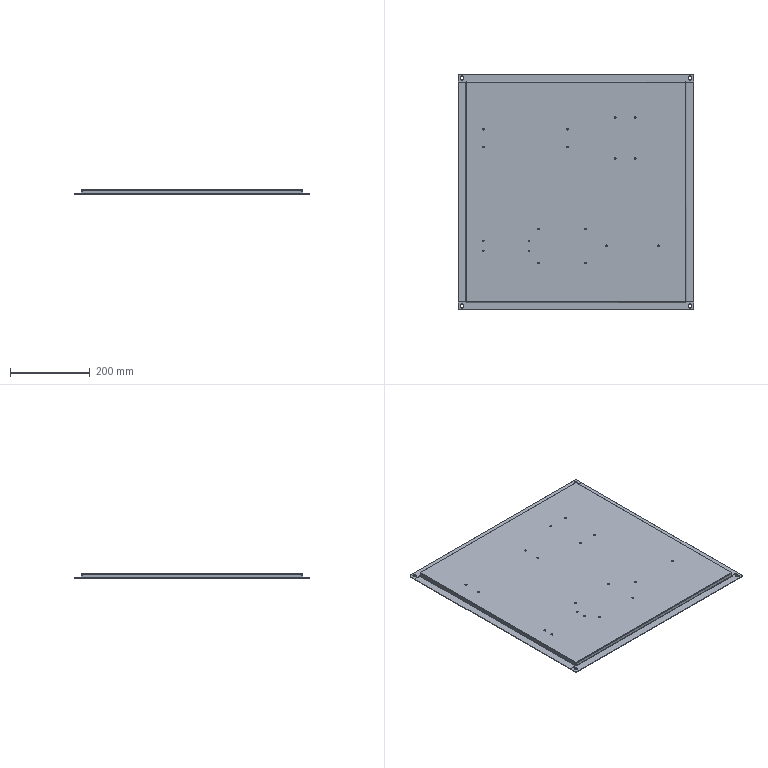Part | SolidWorks | features BaseBody 1 | 1 solid | 294 faces | box 590 x 590 x 11.5 mm | volume 551532 mm3 | plane 190 | cylinder 96 | spline 8 | commonest cylinder face diameters 4 x40 3 x32 1 x8 7 x8 5 x4 10 x4